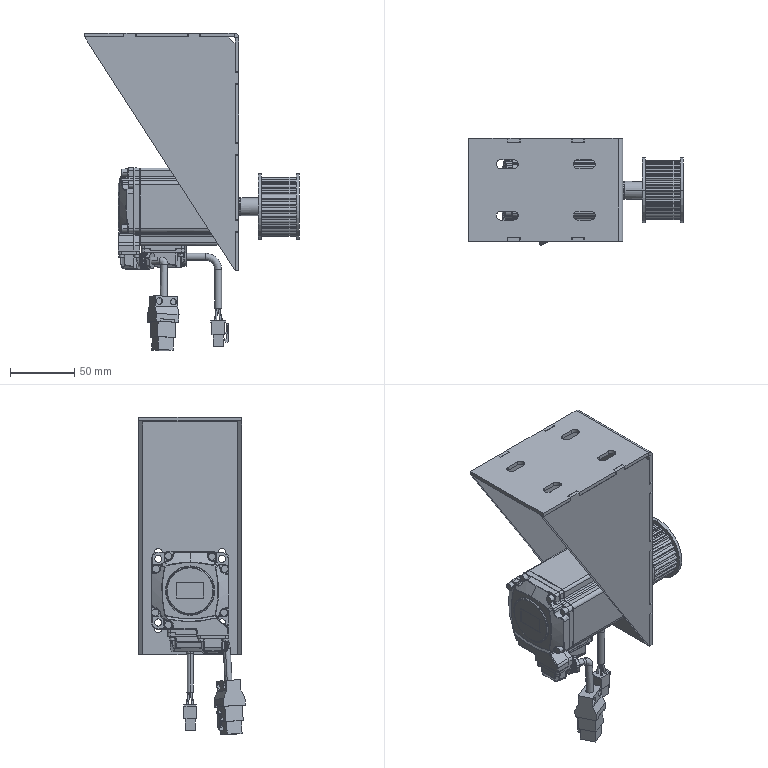Part | 13 solids | 2028 faces | box 167 x 82.945 x 247.154 mm | volume 504890 mm3 | plane 839 | cylinder 697 | cone 185 | spline 153 | torus 126 | sphere 28 | commonest cylinder face diameters 0.4 x134 1 x90 5 x71 4 x47 2 x39 2.5 x39